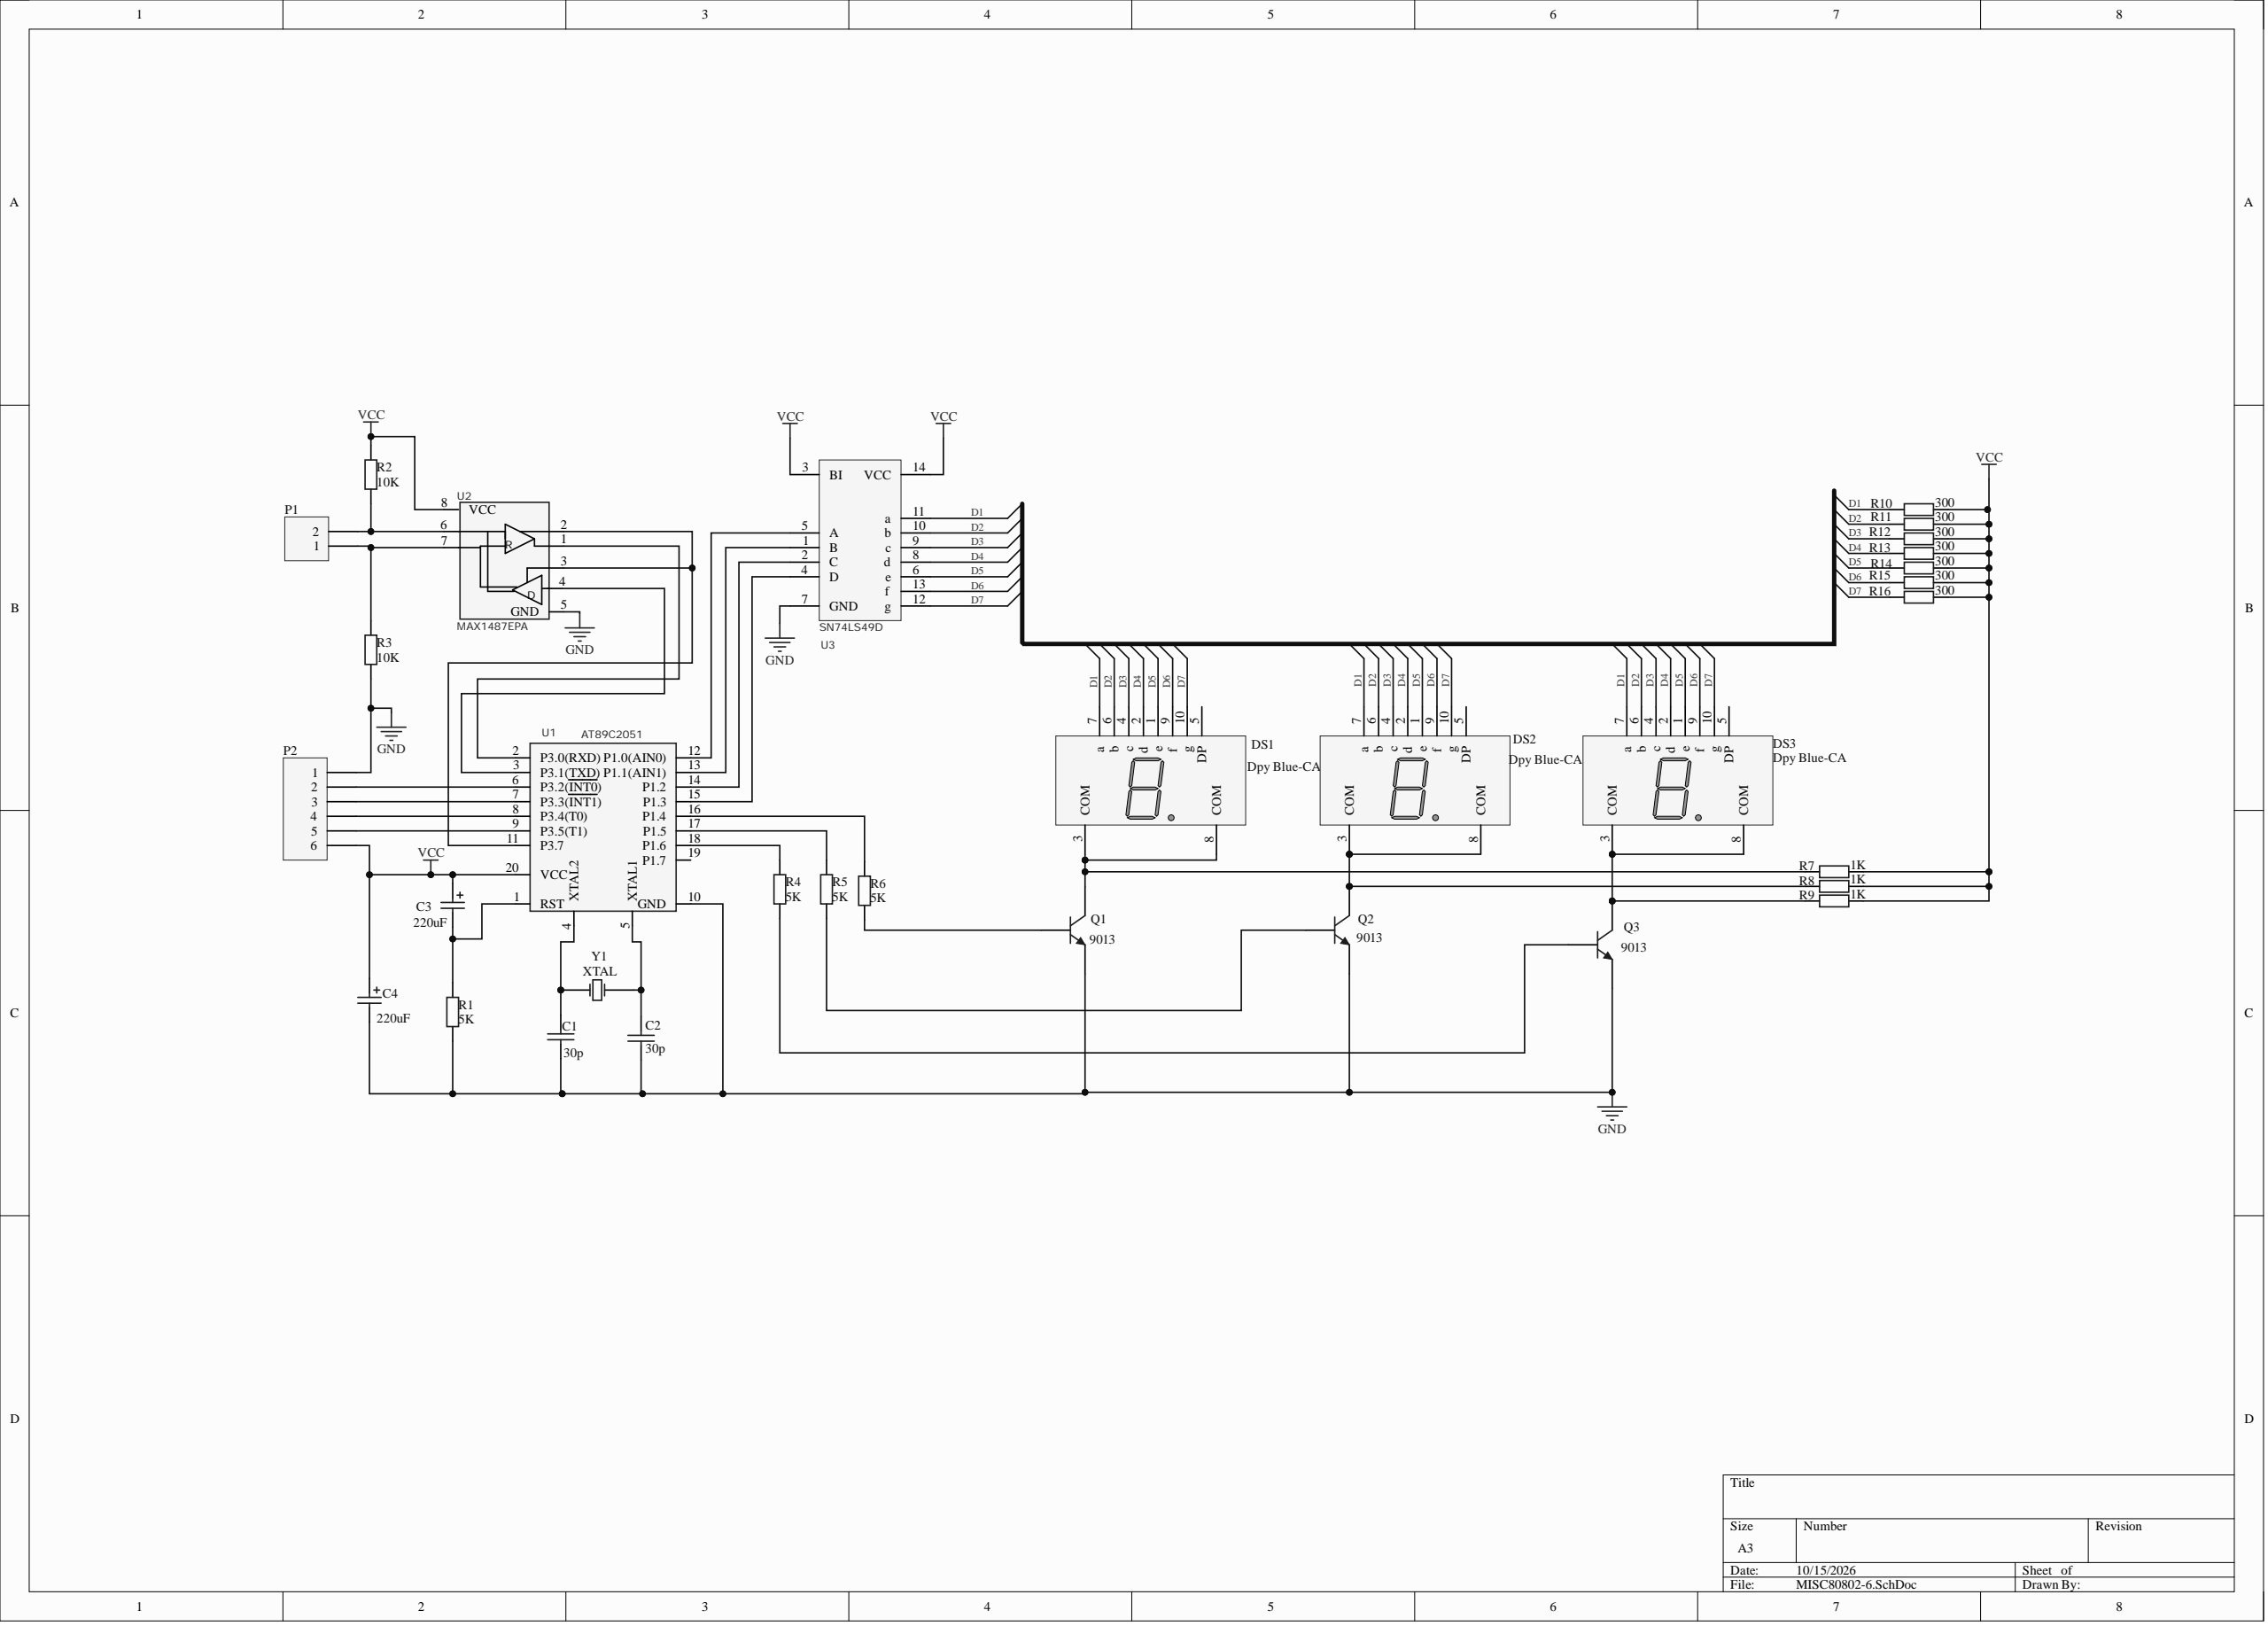Circuit board | Altium Designer | 32 parts | 34 nets
Bill of materials:
Comment,Description,Designator,Footprint,LibRef,Quantity
"30p","","C1, C2","RAD-0.1","瓷片电容","2"
"Cap Pol2","Polarized Capacitor (Axial)","C3","CAPR5-4X5","Cap Pol2","1"
"Cap Pol2","Polarized Capacitor (Axial)","C4","RB5-10.5","Cap Pol2","1"
"Dpy Blue-CA","14.2 mm General Purpose Blue 7-Segment Display: CA, RH DP, Gray Surface","DS1, DS2, DS3","H","Dpy Blue-CA","3"
"Header 2","Header, 2-Pin","P1","HDR1X2","Header 2","1"
"Header 6","Header, 6-Pin","P2","HDR1X6","Header 6","1"
"9013","NPN General Purpose Amplifier","Q1, Q2, Q3","TO-92A","2N3904","3"
"Res2","Resistor","R1, R2, R3, R4, R5, R6, R7, R8, R9, R10, R11, R12, R13, R14, R15, R16","AXIAL-0.4","Res2","16"
"AT89C2051","","U1","DIP20","AT89C2051-24PU","1"
"MAX1487EPA","","U2","PA8","MAX1487EPA","1"
"SN74LS49D","","U3","SOP14","SN74LS49D","1"
"XTAL","Crystal Oscillator","Y1","R38","XTAL","1"
Netlist (Protel format):
[
C1
RAD-0.1
30p



]
[
C2
RAD-0.1
30p



]
[
C3
CAPR5-4X5
Cap Pol2



]
[
C4
RB5-10.5
Cap Pol2



]
[
DS1
H
Dpy Blue-CA



]
[
DS2
H
Dpy Blue-CA



]
[
DS3
H
Dpy Blue-CA



]
[
P1
HDR1X2
Header 2



]
[
P2
HDR1X6
Header 6



]
[
Q1
TO-92A
9013



]
[
Q2
TO-92A
9013



]
[
Q3
TO-92A
9013



]
[
R1
AXIAL-0.4
Res2



]
[
R2
AXIAL-0.4
Res2



]
[
R3
AXIAL-0.4
Res2



]
[
R4
AXIAL-0.4
Res2



]
[
R5
AXIAL-0.4
Res2



]
[
R6
AXIAL-0.4
Res2



]
[
R7
AXIAL-0.4
Res2



]
[
R8
AXIAL-0.4
Res2



]
[
R9
AXIAL-0.4
Res2



]
[
R10
AXIAL-0.4
Res2



]
[
R11
AXIAL-0.4
Res2



]
[
R12
AXIAL-0.4
Res2



]
[
R13
AXIAL-0.4
Res2



]
[
R14
AXIAL-0.4
Res2



]
[
R15
AXIAL-0.4
Res2



]
[
R16
AXIAL-0.4
Res2



]
[
U1
DIP20
AT89C2051



]
[
U2
PA8
MAX1487EPA



]
[
U3
SOP14
SN74LS49D



]
[
Y1
R38
XTAL



]
(
VCC
C3-1
C4-1
P2-6
R2-2
R7-1
R8-1
R9-1
R10-1
R11-1
R12-1
R13-1
R14-1
R15-1
R16-1
U1-20
U2-8
U3-3
U3-14
)
(
NetU1_15
U1-15
U3-4
)
(
NetU1_14
U1-14
U3-2
)
(
NetU1_13
U1-13
U3-1
)
(
NetU1_12
U1-12
U3-5
)
(
NetU1_11
U1-11
U2-2
U2-3
)
(
NetU1_3
U1-3
U2-4
)
(
NetU1_2
U1-2
U2-1
)
(
NetR6_2
R6-2
U1-16
)
(
NetR5_2
R5-2
U1-17
)
(
NetR4_2
R4-2
U1-18
)
(
NetQ3_2
Q3-2
R4-1
)
(
NetQ2_2
Q2-2
R5-1
)
(
NetQ1_2
Q1-2
R6-1
)
(
NetP2_5
P2-5
U1-9
)
(
NetP2_4
P2-4
U1-8
)
(
NetP2_3
P2-3
U1-7
)
(
NetP2_2
P2-2
U1-6
)
(
NetP1_2
P1-2
R2-1
U2-6
)
(
NetP1_1
P1-1
R3-2
U2-7
)
(
NetDS3_3
DS3-3
DS3-8
Q3-3
R9-2
)
(
NetDS2_3
DS2-3
DS2-8
Q2-3
R8-2
)
(
NetDS1_3
DS1-3
DS1-8
Q1-3
R7-2
)
(
NetC3_2
C3-2
R1-2
U1-1
)
(
NetC2_1
C2-1
U1-5
Y1-2
)
(
NetC1_1
C1-1
U1-4
Y1-1
)
(
GND
C1-2
C2-2
C4-2
P2-1
Q1-1
Q2-1
Q3-1
R1-1
R3-1
U1-10
U2-5
U3-7
)
(
D7
DS1-10
DS2-10
DS3-10
R16-2
U3-12
)
(
D6
DS1-9
DS2-9
DS3-9
R15-2
U3-13
)
(
D5
DS1-1
DS2-1
DS3-1
R14-2
U3-6
)
(
D4
DS1-2
DS2-2
DS3-2
R13-2
U3-8
)
(
D3
DS1-4
DS2-4
DS3-4
R12-2
U3-9
)
(
D2
DS1-6
DS2-6
DS3-6
R11-2
U3-10
)
(
D1
DS1-7
DS2-7
DS3-7
R10-2
U3-11
)